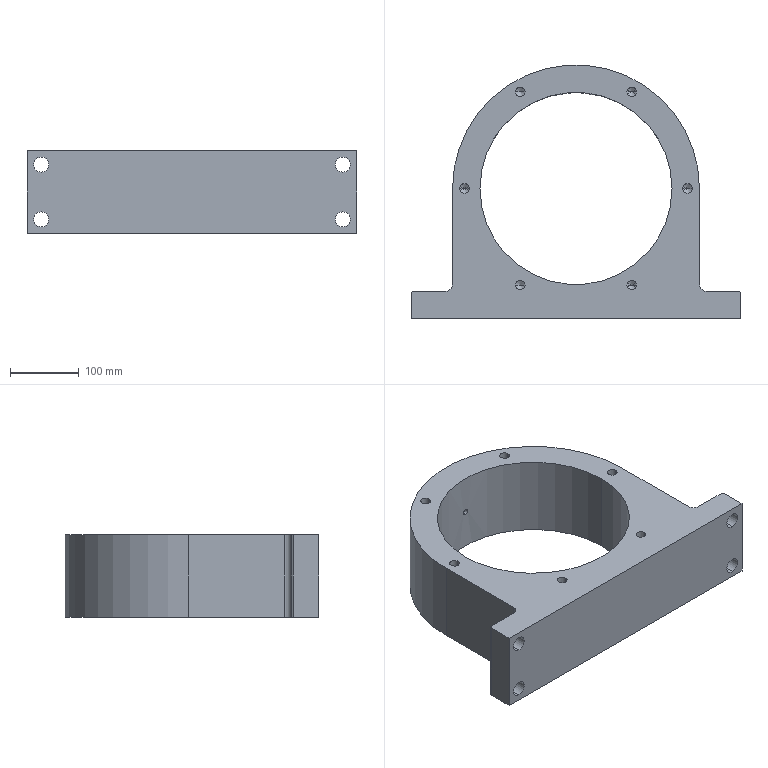Part | SolidWorks | features HoleWzd 3, ICE 2, CirPattern 1, Extrusion 1, Fillet 1, RefAxis 1 | 1 solid | 77 faces | box 480 x 370 x 120 mm | volume 7370776 mm3 | cylinder 43 | cone 24 | plane 10 | commonest cylinder face diameters 14 x24 22 x8 20 x4 6 x2 8.5 x2 280 x2